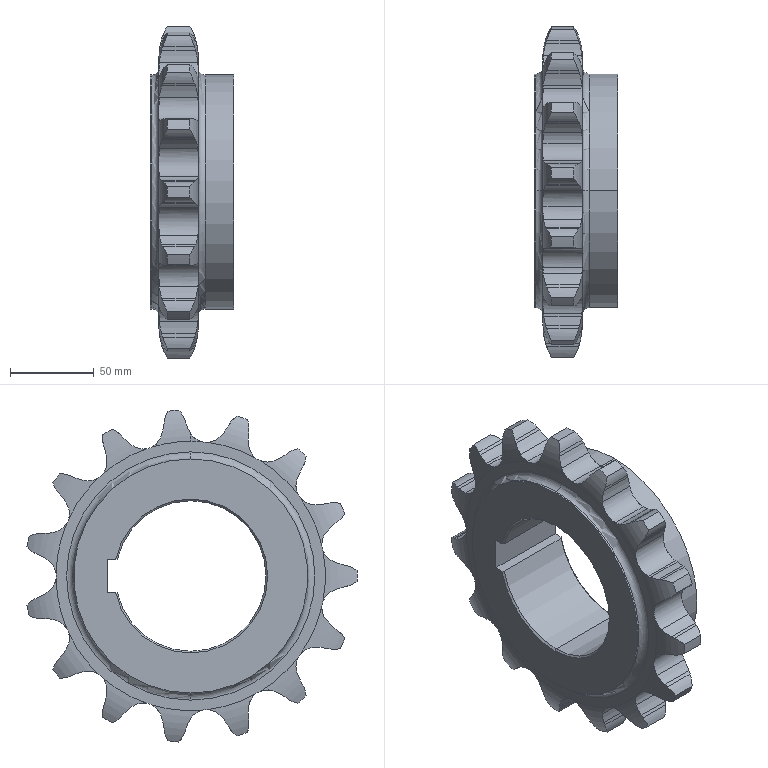Part | SolidWorks | features BaseBody 1 | 1 solid | 183 faces | box 50 x 197.46 x 198.492 mm | volume 656500 mm3 | cylinder 104 | plane 37 | torus 36 | cone 6 | commonest cylinder face diameters 32.838 x32 58.009 x31 22.441 x19 199 x15 140 x4 90 x3